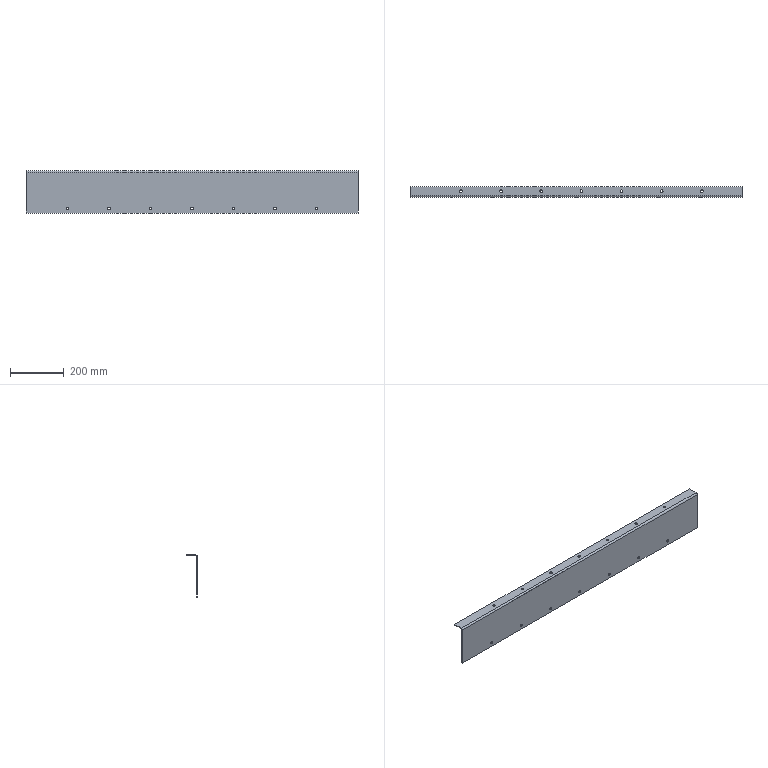Part | SolidWorks | features ICE 2, EdgeFlange 1, FlatPattern 1, SMBaseFlange 1, SheetMetal 1 | 1 solid | 42 faces | box 1240 x 40 x 157 mm | volume 711196 mm3 | cylinder 30 | plane 12 | commonest cylinder face diameters 10 x28 6 x1 12 x1
STEP:
#1=CARTESIAN_POINT('',(475.,20.,78.5));
#2=VERTEX_POINT('',#1);
#3=CARTESIAN_POINT('',(465.,20.,78.5));
#4=VERTEX_POINT('',#3);
#5=CARTESIAN_POINT('',(470.,20.,78.5));
#6=DIRECTION('',(0.,0.,-1.));
#7=DIRECTION('',(-1.,0.,0.));
#8=AXIS2_PLACEMENT_3D('',#5,#6,#7);
#9=CIRCLE('',#8,5.);
#10=EDGE_CURVE('',#2,#4,#9,.T.);
#11=ORIENTED_EDGE('',*,*,#10,.F.);
#12=CARTESIAN_POINT('',(475.,20.,75.5));
#13=VERTEX_POINT('',#12);
#14=CARTESIAN_POINT('',(475.,20.,255.5));
#15=DIRECTION('',(0.,0.,-1.));
#16=VECTOR('',#15,1000.);
#17=LINE('',#14,#16);
#18=EDGE_CURVE('',#2,#13,#17,.T.);
#19=ORIENTED_EDGE('',*,*,#18,.T.);
#20=CARTESIAN_POINT('',(465.,20.,75.5));
#21=VERTEX_POINT('',#20);
#22=CARTESIAN_POINT('',(470.,20.,75.5));
#23=DIRECTION('',(0.,0.,-1.));
#24=DIRECTION('',(-1.,0.,0.));
#25=AXIS2_PLACEMENT_3D('',#22,#23,#24);
#26=CIRCLE('',#25,5.);
#27=EDGE_CURVE('',#13,#21,#26,.T.);
#28=ORIENTED_EDGE('',*,*,#27,.T.);
#29=CARTESIAN_POINT('',(465.,20.,255.5));
#30=DIRECTION('',(0.,0.,-1.));
#31=VECTOR('',#30,1000.);
#32=LINE('',#29,#31);
#33=EDGE_CURVE('',#4,#21,#32,.T.);
#34=ORIENTED_EDGE('',*,*,#33,.F.);
#35=EDGE_LOOP('',(#11,#19,#28,#34));
#36=FACE_OUTER_BOUND('',#35,.T.);
#37=CARTESIAN_POINT('',(470.,20.,255.5));
#38=DIRECTION('',(0.,0.,-1.));
#39=DIRECTION('',(-1.,0.,0.));
#40=AXIS2_PLACEMENT_3D('',#37,#38,#39);
#41=CYLINDRICAL_SURFACE('',#40,5.);
#42=ADVANCED_FACE('',(#36),#41,.F.);
#43=CARTESIAN_POINT('',(325.,20.,78.5));
#44=VERTEX_POINT('',#43);
#45=CARTESIAN_POINT('',(315.,20.,78.5));
#46=VERTEX_POINT('',#45);
#47=CARTESIAN_POINT('',(320.,20.,78.5));
#48=DIRECTION('',(0.,0.,-1.));
#49=DIRECTION('',(-1.,0.,0.));
#50=AXIS2_PLACEMENT_3D('',#47,#48,#49);
#51=CIRCLE('',#50,5.);
#52=EDGE_CURVE('',#44,#46,#51,.T.);
#53=ORIENTED_EDGE('',*,*,#52,.F.);
#54=CARTESIAN_POINT('',(325.,20.,75.5));
#55=VERTEX_POINT('',#54);
#56=CARTESIAN_POINT('',(325.,20.,255.5));
#57=DIRECTION('',(0.,0.,-1.));
#58=VECTOR('',#57,1000.);
#59=LINE('',#56,#58);
#60=EDGE_CURVE('',#44,#55,#59,.T.);
#61=ORIENTED_EDGE('',*,*,#60,.T.);
#62=CARTESIAN_POINT('',(315.,20.,75.5));
#63=VERTEX_POINT('',#62);
#64=CARTESIAN_POINT('',(320.,20.,75.5));
#65=DIRECTION('',(0.,0.,-1.));
#66=DIRECTION('',(-1.,0.,0.));
#67=AXIS2_PLACEMENT_3D('',#64,#65,#66);
#68=CIRCLE('',#67,5.);
#69=EDGE_CURVE('',#55,#63,#68,.T.);
#70=ORIENTED_EDGE('',*,*,#69,.T.);
#71=CARTESIAN_POINT('',(315.,20.,255.5));
#72=DIRECTION('',(0.,0.,-1.));
#73=VECTOR('',#72,1000.);
#74=LINE('',#71,#73);
#75=EDGE_CURVE('',#46,#63,#74,.T.);
#76=ORIENTED_EDGE('',*,*,#75,.F.);
#77=EDGE_LOOP('',(#53,#61,#70,#76));
#78=FACE_OUTER_BOUND('',#77,.T.);
#79=CARTESIAN_POINT('',(320.,20.,255.5));
#80=DIRECTION('',(0.,0.,-1.));
#81=DIRECTION('',(-1.,0.,0.));
#82=AXIS2_PLACEMENT_3D('',#79,#80,#81);
#83=CYLINDRICAL_SURFACE('',#82,5.);
#84=ADVANCED_FACE('',(#78),#83,.F.);
#85=CARTESIAN_POINT('',(175.,20.,78.5));
#86=VERTEX_POINT('',#85);
#87=CARTESIAN_POINT('',(165.,20.,78.5));
#88=VERTEX_POINT('',#87);
#89=CARTESIAN_POINT('',(170.,20.,78.5));
#90=DIRECTION('',(0.,0.,-1.));
#91=DIRECTION('',(-1.,0.,0.));
#92=AXIS2_PLACEMENT_3D('',#89,#90,#91);
#93=CIRCLE('',#92,5.);
#94=EDGE_CURVE('',#86,#88,#93,.T.);
#95=ORIENTED_EDGE('',*,*,#94,.F.);
#96=CARTESIAN_POINT('',(175.,20.,75.5));
#97=VERTEX_POINT('',#96);
#98=CARTESIAN_POINT('',(175.,20.,255.5));
#99=DIRECTION('',(0.,0.,-1.));
#100=VECTOR('',#99,1000.);
#101=LINE('',#98,#100);
#102=EDGE_CURVE('',#86,#97,#101,.T.);
#103=ORIENTED_EDGE('',*,*,#102,.T.);
#104=CARTESIAN_POINT('',(165.,20.,75.5));
#105=VERTEX_POINT('',#104);
#106=CARTESIAN_POINT('',(170.,20.,75.5));
#107=DIRECTION('',(0.,0.,-1.));
#108=DIRECTION('',(-1.,0.,0.));
#109=AXIS2_PLACEMENT_3D('',#106,#107,#108);
#110=CIRCLE('',#109,5.);
#111=EDGE_CURVE('',#97,#105,#110,.T.);
#112=ORIENTED_EDGE('',*,*,#111,.T.);
#113=CARTESIAN_POINT('',(165.,20.,255.5));
#114=DIRECTION('',(0.,0.,-1.));
#115=VECTOR('',#114,1000.);
#116=LINE('',#113,#115);
#117=EDGE_CURVE('',#88,#105,#116,.T.);
#118=ORIENTED_EDGE('',*,*,#117,.F.);
#119=EDGE_LOOP('',(#95,#103,#112,#118));
#120=FACE_OUTER_BOUND('',#119,.T.);
#121=CARTESIAN_POINT('',(170.,20.,255.5));
#122=DIRECTION('',(0.,0.,-1.));
#123=DIRECTION('',(-1.,0.,0.));
#124=AXIS2_PLACEMENT_3D('',#121,#122,#123);
#125=CYLINDRICAL_SURFACE('',#124,5.);
#126=ADVANCED_FACE('',(#120),#125,.F.);
#127=CARTESIAN_POINT('',(25.,20.,78.5));
#128=VERTEX_POINT('',#127);
#129=CARTESIAN_POINT('',(15.,20.,78.5));
#130=VERTEX_POINT('',#129);
#131=CARTESIAN_POINT('',(20.,20.,78.5));
#132=DIRECTION('',(0.,0.,-1.));
#133=DIRECTION('',(-1.,0.,0.));
#134=AXIS2_PLACEMENT_3D('',#131,#132,#133);
#135=CIRCLE('',#134,5.);
#136=EDGE_CURVE('',#128,#130,#135,.T.);
#137=ORIENTED_EDGE('',*,*,#136,.F.);
#138=CARTESIAN_POINT('',(25.,20.,75.5));
#139=VERTEX_POINT('',#138);
#140=CARTESIAN_POINT('',(25.,20.,255.5));
#141=DIRECTION('',(0.,0.,-1.));
#142=VECTOR('',#141,1000.);
#143=LINE('',#140,#142);
#144=EDGE_CURVE('',#128,#139,#143,.T.);
#145=ORIENTED_EDGE('',*,*,#144,.T.);
#146=CARTESIAN_POINT('',(15.,20.,75.5));
#147=VERTEX_POINT('',#146);
#148=CARTESIAN_POINT('',(20.,20.,75.5));
#149=DIRECTION('',(0.,0.,-1.));
#150=DIRECTION('',(-1.,0.,0.));
#151=AXIS2_PLACEMENT_3D('',#148,#149,#150);
#152=CIRCLE('',#151,5.);
#153=EDGE_CURVE('',#139,#147,#152,.T.);
#154=ORIENTED_EDGE('',*,*,#153,.T.);
#155=CARTESIAN_POINT('',(15.,20.,255.5));
#156=DIRECTION('',(0.,0.,-1.));
#157=VECTOR('',#156,1000.);
#158=LINE('',#155,#157);
#159=EDGE_CURVE('',#130,#147,#158,.T.);
#160=ORIENTED_EDGE('',*,*,#159,.F.);
#161=EDGE_LOOP('',(#137,#145,#154,#160));
#162=FACE_OUTER_BOUND('',#161,.T.);
#163=CARTESIAN_POINT('',(20.,20.,255.5));
#164=DIRECTION('',(0.,0.,-1.));
#165=DIRECTION('',(-1.,0.,0.));
#166=AXIS2_PLACEMENT_3D('',#163,#164,#165);
#167=CYLINDRICAL_SURFACE('',#166,5.);
#168=ADVANCED_FACE('',(#162),#167,.F.);
#169=CARTESIAN_POINT('',(-125.,20.,78.5));
#170=VERTEX_POINT('',#169);
#171=CARTESIAN_POINT('',(-135.,20.,78.5));
#172=VERTEX_POINT('',#171);
#173=CARTESIAN_POINT('',(-130.,20.,78.5));
#174=DIRECTION('',(0.,0.,-1.));
#175=DIRECTION('',(-1.,0.,0.));
#176=AXIS2_PLACEMENT_3D('',#173,#174,#175);
#177=CIRCLE('',#176,5.);
#178=EDGE_CURVE('',#170,#172,#177,.T.);
#179=ORIENTED_EDGE('',*,*,#178,.F.);
#180=CARTESIAN_POINT('',(-125.,20.,75.5));
#181=VERTEX_POINT('',#180);
#182=CARTESIAN_POINT('',(-125.,20.,255.5));
#183=DIRECTION('',(0.,0.,-1.));
#184=VECTOR('',#183,1000.);
#185=LINE('',#182,#184);
#186=EDGE_CURVE('',#170,#181,#185,.T.);
#187=ORIENTED_EDGE('',*,*,#186,.T.);
#188=CARTESIAN_POINT('',(-135.,20.,75.5));
#189=VERTEX_POINT('',#188);
#190=CARTESIAN_POINT('',(-130.,20.,75.5));
#191=DIRECTION('',(0.,0.,-1.));
#192=DIRECTION('',(-1.,0.,0.));
#193=AXIS2_PLACEMENT_3D('',#190,#191,#192);
#194=CIRCLE('',#193,5.);
#195=EDGE_CURVE('',#181,#189,#194,.T.);
#196=ORIENTED_EDGE('',*,*,#195,.T.);
#197=CARTESIAN_POINT('',(-135.,20.,255.5));
#198=DIRECTION('',(0.,0.,-1.));
#199=VECTOR('',#198,1000.);
#200=LINE('',#197,#199);
#201=EDGE_CURVE('',#172,#189,#200,.T.);
#202=ORIENTED_EDGE('',*,*,#201,.F.);
#203=EDGE_LOOP('',(#179,#187,#196,#202));
#204=FACE_OUTER_BOUND('',#203,.T.);
#205=CARTESIAN_POINT('',(-130.,20.,255.5));
#206=DIRECTION('',(0.,0.,-1.));
#207=DIRECTION('',(-1.,0.,0.));
#208=AXIS2_PLACEMENT_3D('',#205,#206,#207);
#209=CYLINDRICAL_SURFACE('',#208,5.);
#210=ADVANCED_FACE('',(#204),#209,.F.);
#211=CARTESIAN_POINT('',(-275.,20.,78.5));
#212=VERTEX_POINT('',#211);
#213=CARTESIAN_POINT('',(-285.,20.,78.5));
#214=VERTEX_POINT('',#213);
#215=CARTESIAN_POINT('',(-280.,20.,78.5));
#216=DIRECTION('',(0.,0.,-1.));
#217=DIRECTION('',(-1.,0.,0.));
#218=AXIS2_PLACEMENT_3D('',#215,#216,#217);
#219=CIRCLE('',#218,5.);
#220=EDGE_CURVE('',#212,#214,#219,.T.);
#221=ORIENTED_EDGE('',*,*,#220,.F.);
#222=CARTESIAN_POINT('',(-275.,20.,75.5));
#223=VERTEX_POINT('',#222);
#224=CARTESIAN_POINT('',(-275.,20.,255.5));
#225=DIRECTION('',(0.,0.,-1.));
#226=VECTOR('',#225,1000.);
#227=LINE('',#224,#226);
#228=EDGE_CURVE('',#212,#223,#227,.T.);
#229=ORIENTED_EDGE('',*,*,#228,.T.);
#230=CARTESIAN_POINT('',(-285.,20.,75.5));
#231=VERTEX_POINT('',#230);
#232=CARTESIAN_POINT('',(-280.,20.,75.5));
#233=DIRECTION('',(0.,0.,-1.));
#234=DIRECTION('',(-1.,0.,0.));
#235=AXIS2_PLACEMENT_3D('',#232,#233,#234);
#236=CIRCLE('',#235,5.);
#237=EDGE_CURVE('',#223,#231,#236,.T.);
#238=ORIENTED_EDGE('',*,*,#237,.T.);
#239=CARTESIAN_POINT('',(-285.,20.,255.5));
#240=DIRECTION('',(0.,0.,-1.));
#241=VECTOR('',#240,1000.);
#242=LINE('',#239,#241);
#243=EDGE_CURVE('',#214,#231,#242,.T.);
#244=ORIENTED_EDGE('',*,*,#243,.F.);
#245=EDGE_LOOP('',(#221,#229,#238,#244));
#246=FACE_OUTER_BOUND('',#245,.T.);
#247=CARTESIAN_POINT('',(-280.,20.,255.5));
#248=DIRECTION('',(0.,0.,-1.));
#249=DIRECTION('',(-1.,0.,0.));
#250=AXIS2_PLACEMENT_3D('',#247,#248,#249);
#251=CYLINDRICAL_SURFACE('',#250,5.);
#252=ADVANCED_FACE('',(#246),#251,.F.);
#253=CARTESIAN_POINT('',(-425.,20.,78.5));
#254=VERTEX_POINT('',#253);
#255=CARTESIAN_POINT('',(-435.,20.,78.5));
#256=VERTEX_POINT('',#255);
#257=CARTESIAN_POINT('',(-430.,20.,78.5));
#258=DIRECTION('',(0.,0.,-1.));
#259=DIRECTION('',(-1.,0.,0.));
#260=AXIS2_PLACEMENT_3D('',#257,#258,#259);
#261=CIRCLE('',#260,5.);
#262=EDGE_CURVE('',#254,#256,#261,.T.);
#263=ORIENTED_EDGE('',*,*,#262,.F.);
#264=CARTESIAN_POINT('',(-425.,20.,75.5));
#265=VERTEX_POINT('',#264);
#266=CARTESIAN_POINT('',(-425.,20.,255.5));
#267=DIRECTION('',(0.,0.,-1.));
#268=VECTOR('',#267,1000.);
#269=LINE('',#266,#268);
#270=EDGE_CURVE('',#254,#265,#269,.T.);
#271=ORIENTED_EDGE('',*,*,#270,.T.);
#272=CARTESIAN_POINT('',(-435.,20.,75.5));
#273=VERTEX_POINT('',#272);
#274=CARTESIAN_POINT('',(-430.,20.,75.5));
#275=DIRECTION('',(0.,0.,-1.));
#276=DIRECTION('',(-1.,0.,0.));
#277=AXIS2_PLACEMENT_3D('',#274,#275,#276);
#278=CIRCLE('',#277,5.);
#279=EDGE_CURVE('',#265,#273,#278,.T.);
#280=ORIENTED_EDGE('',*,*,#279,.T.);
#281=CARTESIAN_POINT('',(-435.,20.,255.5));
#282=DIRECTION('',(0.,0.,-1.));
#283=VECTOR('',#282,1000.);
#284=LINE('',#281,#283);
#285=EDGE_CURVE('',#256,#273,#284,.T.);
#286=ORIENTED_EDGE('',*,*,#285,.F.);
#287=EDGE_LOOP('',(#263,#271,#280,#286));
#288=FACE_OUTER_BOUND('',#287,.T.);
#289=CARTESIAN_POINT('',(-430.,20.,255.5));
#290=DIRECTION('',(0.,0.,-1.));
#291=DIRECTION('',(-1.,0.,0.));
#292=AXIS2_PLACEMENT_3D('',#289,#290,#291);
#293=CYLINDRICAL_SURFACE('',#292,5.);
#294=ADVANCED_FACE('',(#288),#293,.F.);
#295=CARTESIAN_POINT('',(465.,-3.,-66.5));
#296=VERTEX_POINT('',#295);
#297=CARTESIAN_POINT('',(465.,-3.,-56.5));
#298=VERTEX_POINT('',#297);
#299=CARTESIAN_POINT('',(465.,-3.,-61.5));
#300=DIRECTION('',(0.,1.,0.));
#301=DIRECTION('',(0.,0.,1.));
#302=AXIS2_PLACEMENT_3D('',#299,#300,#301);
#303=CIRCLE('',#302,5.);
#304=EDGE_CURVE('',#296,#298,#303,.T.);
#305=ORIENTED_EDGE('',*,*,#304,.F.);
#306=CARTESIAN_POINT('',(465.,0.,-66.5));
#307=VERTEX_POINT('',#306);
#308=CARTESIAN_POINT('',(465.,-54.,-66.5));
#309=DIRECTION('',(0.,1.,0.));
#310=VECTOR('',#309,1000.);
#311=LINE('',#308,#310);
#312=EDGE_CURVE('',#296,#307,#311,.T.);
#313=ORIENTED_EDGE('',*,*,#312,.T.);
#314=CARTESIAN_POINT('',(465.,0.,-56.5));
#315=VERTEX_POINT('',#314);
#316=CARTESIAN_POINT('',(465.,0.,-61.5));
#317=DIRECTION('',(0.,1.,0.));
#318=DIRECTION('',(0.,0.,1.));
#319=AXIS2_PLACEMENT_3D('',#316,#317,#318);
#320=CIRCLE('',#319,5.);
#321=EDGE_CURVE('',#307,#315,#320,.T.);
#322=ORIENTED_EDGE('',*,*,#321,.T.);
#323=CARTESIAN_POINT('',(465.,-54.,-56.5));
#324=DIRECTION('',(0.,1.,0.));
#325=VECTOR('',#324,1000.);
#326=LINE('',#323,#325);
#327=EDGE_CURVE('',#298,#315,#326,.T.);
#328=ORIENTED_EDGE('',*,*,#327,.F.);
#329=EDGE_LOOP('',(#305,#313,#322,#328));
#330=FACE_OUTER_BOUND('',#329,.T.);
#331=CARTESIAN_POINT('',(465.,-54.,-61.5));
#332=DIRECTION('',(0.,1.,0.));
#333=DIRECTION('',(0.,0.,1.));
#334=AXIS2_PLACEMENT_3D('',#331,#332,#333);
#335=CYLINDRICAL_SURFACE('',#334,5.);
#336=ADVANCED_FACE('',(#330),#335,.F.);
#337=CARTESIAN_POINT('',(310.,-3.,-66.5));
#338=VERTEX_POINT('',#337);
#339=CARTESIAN_POINT('',(310.,-3.,-56.5));
#340=VERTEX_POINT('',#339);
#341=CARTESIAN_POINT('',(310.,-3.,-61.5));
#342=DIRECTION('',(0.,1.,0.));
#343=DIRECTION('',(0.,0.,1.));
#344=AXIS2_PLACEMENT_3D('',#341,#342,#343);
#345=CIRCLE('',#344,5.);
#346=EDGE_CURVE('',#338,#340,#345,.T.);
#347=ORIENTED_EDGE('',*,*,#346,.F.);
#348=CARTESIAN_POINT('',(310.,0.,-66.5));
#349=VERTEX_POINT('',#348);
#350=CARTESIAN_POINT('',(310.,-54.,-66.5));
#351=DIRECTION('',(0.,1.,0.));
#352=VECTOR('',#351,1000.);
#353=LINE('',#350,#352);
#354=EDGE_CURVE('',#338,#349,#353,.T.);
#355=ORIENTED_EDGE('',*,*,#354,.T.);
#356=CARTESIAN_POINT('',(310.,0.,-56.5));
#357=VERTEX_POINT('',#356);
#358=CARTESIAN_POINT('',(310.,0.,-61.5));
#359=DIRECTION('',(0.,1.,0.));
#360=DIRECTION('',(0.,0.,1.));
#361=AXIS2_PLACEMENT_3D('',#358,#359,#360);
#362=CIRCLE('',#361,5.);
#363=EDGE_CURVE('',#349,#357,#362,.T.);
#364=ORIENTED_EDGE('',*,*,#363,.T.);
#365=CARTESIAN_POINT('',(310.,-54.,-56.5));
#366=DIRECTION('',(0.,1.,0.));
#367=VECTOR('',#366,1000.);
#368=LINE('',#365,#367);
#369=EDGE_CURVE('',#340,#357,#368,.T.);
#370=ORIENTED_EDGE('',*,*,#369,.F.);
#371=EDGE_LOOP('',(#347,#355,#364,#370));
#372=FACE_OUTER_BOUND('',#371,.T.);
#373=CARTESIAN_POINT('',(310.,-54.,-61.5));
#374=DIRECTION('',(0.,1.,0.));
#375=DIRECTION('',(0.,0.,1.));
#376=AXIS2_PLACEMENT_3D('',#373,#374,#375);
#377=CYLINDRICAL_SURFACE('',#376,5.);
#378=ADVANCED_FACE('',(#372),#377,.F.);
#379=CARTESIAN_POINT('',(155.,-3.,-66.5));
#380=VERTEX_POINT('',#379);
#381=CARTESIAN_POINT('',(155.,-3.,-56.5));
#382=VERTEX_POINT('',#381);
#383=CARTESIAN_POINT('',(155.,-3.,-61.5));
#384=DIRECTION('',(0.,1.,0.));
#385=DIRECTION('',(0.,0.,1.));
#386=AXIS2_PLACEMENT_3D('',#383,#384,#385);
#387=CIRCLE('',#386,5.);
#388=EDGE_CURVE('',#380,#382,#387,.T.);
#389=ORIENTED_EDGE('',*,*,#388,.F.);
#390=CARTESIAN_POINT('',(155.,0.,-66.5));
#391=VERTEX_POINT('',#390);
#392=CARTESIAN_POINT('',(155.,-54.,-66.5));
#393=DIRECTION('',(0.,1.,0.));
#394=VECTOR('',#393,1000.);
#395=LINE('',#392,#394);
#396=EDGE_CURVE('',#380,#391,#395,.T.);
#397=ORIENTED_EDGE('',*,*,#396,.T.);
#398=CARTESIAN_POINT('',(155.,0.,-56.5));
#399=VERTEX_POINT('',#398);
#400=CARTESIAN_POINT('',(155.,0.,-61.5));
#401=DIRECTION('',(0.,1.,0.));
#402=DIRECTION('',(0.,0.,1.));
#403=AXIS2_PLACEMENT_3D('',#400,#401,#402);
#404=CIRCLE('',#403,5.);
#405=EDGE_CURVE('',#391,#399,#404,.T.);
#406=ORIENTED_EDGE('',*,*,#405,.T.);
#407=CARTESIAN_POINT('',(155.,-54.,-56.5));
#408=DIRECTION('',(0.,1.,0.));
#409=VECTOR('',#408,1000.);
#410=LINE('',#407,#409);
#411=EDGE_CURVE('',#382,#399,#410,.T.);
#412=ORIENTED_EDGE('',*,*,#411,.F.);
#413=EDGE_LOOP('',(#389,#397,#406,#412));
#414=FACE_OUTER_BOUND('',#413,.T.);
#415=CARTESIAN_POINT('',(155.,-54.,-61.5));
#416=DIRECTION('',(0.,1.,0.));
#417=DIRECTION('',(0.,0.,1.));
#418=AXIS2_PLACEMENT_3D('',#415,#416,#417);
#419=CYLINDRICAL_SURFACE('',#418,5.);
#420=ADVANCED_FACE('',(#414),#419,.F.);
#421=CARTESIAN_POINT('',(0.,-3.,-66.5));
#422=VERTEX_POINT('',#421);
#423=CARTESIAN_POINT('',(0.,-3.,-56.5));
#424=VERTEX_POINT('',#423);
#425=CARTESIAN_POINT('',(0.,-3.,-61.5));
#426=DIRECTION('',(0.,1.,0.));
#427=DIRECTION('',(0.,0.,1.));
#428=AXIS2_PLACEMENT_3D('',#425,#426,#427);
#429=CIRCLE('',#428,5.);
#430=EDGE_CURVE('',#422,#424,#429,.T.);
#431=ORIENTED_EDGE('',*,*,#430,.F.);
#432=CARTESIAN_POINT('',(0.,0.,-66.5));
#433=VERTEX_POINT('',#432);
#434=CARTESIAN_POINT('',(0.,-54.,-66.5));
#435=DIRECTION('',(0.,1.,0.));
#436=VECTOR('',#435,1000.);
#437=LINE('',#434,#436);
#438=EDGE_CURVE('',#422,#433,#437,.T.);
#439=ORIENTED_EDGE('',*,*,#438,.T.);
#440=CARTESIAN_POINT('',(0.,0.,-56.5));
#441=VERTEX_POINT('',#440);
#442=CARTESIAN_POINT('',(0.,0.,-61.5));
#443=DIRECTION('',(0.,1.,0.));
#444=DIRECTION('',(0.,0.,1.));
#445=AXIS2_PLACEMENT_3D('',#442,#443,#444);
#446=CIRCLE('',#445,5.);
#447=EDGE_CURVE('',#433,#441,#446,.T.);
#448=ORIENTED_EDGE('',*,*,#447,.T.);
#449=CARTESIAN_POINT('',(0.,-54.,-56.5));
#450=DIRECTION('',(0.,1.,0.));
#451=VECTOR('',#450,1000.);
#452=LINE('',#449,#451);
#453=EDGE_CURVE('',#424,#441,#452,.T.);
#454=ORIENTED_EDGE('',*,*,#453,.F.);
#455=EDGE_LOOP('',(#431,#439,#448,#454));
#456=FACE_OUTER_BOUND('',#455,.T.);
#457=CARTESIAN_POINT('',(0.,-54.,-61.5));
#458=DIRECTION('',(0.,1.,0.));
#459=DIRECTION('',(0.,0.,1.));
#460=AXIS2_PLACEMENT_3D('',#457,#458,#459);
#461=CYLINDRICAL_SURFACE('',#460,5.);
#462=ADVANCED_FACE('',(#456),#461,.F.);
#463=CARTESIAN_POINT('',(-155.,-3.,-66.5));
#464=VERTEX_POINT('',#463);
#465=CARTESIAN_POINT('',(-155.,-3.,-56.5));
#466=VERTEX_POINT('',#465);
#467=CARTESIAN_POINT('',(-155.,-3.,-61.5));
#468=DIRECTION('',(0.,1.,0.));
#469=DIRECTION('',(0.,0.,1.));
#470=AXIS2_PLACEMENT_3D('',#467,#468,#469);
#471=CIRCLE('',#470,5.);
#472=EDGE_CURVE('',#464,#466,#471,.T.);
#473=ORIENTED_EDGE('',*,*,#472,.F.);
#474=CARTESIAN_POINT('',(-155.,0.,-66.5));
#475=VERTEX_POINT('',#474);
#476=CARTESIAN_POINT('',(-155.,-54.,-66.5));
#477=DIRECTION('',(0.,1.,0.));
#478=VECTOR('',#477,1000.);
#479=LINE('',#476,#478);
#480=EDGE_CURVE('',#464,#475,#479,.T.);
#481=ORIENTED_EDGE('',*,*,#480,.T.);
#482=CARTESIAN_POINT('',(-155.,0.,-56.5));
#483=VERTEX_POINT('',#482);
#484=CARTESIAN_POINT('',(-155.,0.,-61.5));
#485=DIRECTION('',(0.,1.,0.));
#486=DIRECTION('',(0.,0.,1.));
#487=AXIS2_PLACEMENT_3D('',#484,#485,#486);
#488=CIRCLE('',#487,5.);
#489=EDGE_CURVE('',#475,#483,#488,.T.);
#490=ORIENTED_EDGE('',*,*,#489,.T.);
#491=CARTESIAN_POINT('',(-155.,-54.,-56.5));
#492=DIRECTION('',(0.,1.,0.));
#493=VECTOR('',#492,1000.);
#494=LINE('',#491,#493);
#495=EDGE_CURVE('',#466,#483,#494,.T.);
#496=ORIENTED_EDGE('',*,*,#495,.F.);
#497=EDGE_LOOP('',(#473,#481,#490,#496));
#498=FACE_OUTER_BOUND('',#497,.T.);
#499=CARTESIAN_POINT('',(-155.,-54.,-61.5));
#500=DIRECTION('',(0.,1.,0.));
#501=DIRECTION('',(0.,0.,1.));
#502=AXIS2_PLACEMENT_3D('',#499,#500,#501);
#503=CYLINDRICAL_SURFACE('',#502,5.);
#504=ADVANCED_FACE('',(#498),#503,.F.);
#505=CARTESIAN_POINT('',(-310.,-3.,-66.5));
#506=VERTEX_POINT('',#505);
#507=CARTESIAN_POINT('',(-310.,-3.,-56.5));
#508=VERTEX_POINT('',#507);
#509=CARTESIAN_POINT('',(-310.,-3.,-61.5));
#510=DIRECTION('',(0.,1.,0.));
#511=DIRECTION('',(0.,0.,1.));
#512=AXIS2_PLACEMENT_3D('',#509,#510,#511);
#513=CIRCLE('',#512,5.);
#514=EDGE_CURVE('',#506,#508,#513,.T.);
#515=ORIENTED_EDGE('',*,*,#514,.F.);
#516=CARTESIAN_POINT('',(-310.,0.,-66.5));
#517=VERTEX_POINT('',#516);
#518=CARTESIAN_POINT('',(-310.,-54.,-66.5));
#519=DIRECTION('',(0.,1.,0.));
#520=VECTOR('',#519,1000.);
#521=LINE('',#518,#520);
#522=EDGE_CURVE('',#506,#517,#521,.T.);
#523=ORIENTED_EDGE('',*,*,#522,.T.);
#524=CARTESIAN_POINT('',(-310.,0.,-56.5));
#525=VERTEX_POINT('',#524);
#526=CARTESIAN_POINT('',(-310.,0.,-61.5));
#527=DIRECTION('',(0.,1.,0.));
#528=DIRECTION('',(0.,0.,1.));
#529=AXIS2_PLACEMENT_3D('',#526,#527,#528);
#530=CIRCLE('',#529,5.);
#531=EDGE_CURVE('',#517,#525,#530,.T.);
#532=ORIENTED_EDGE('',*,*,#531,.T.);
#533=CARTESIAN_POINT('',(-310.,-54.,-56.5));
#534=DIRECTION('',(0.,1.,0.));
#535=VECTOR('',#534,1000.);
#536=LINE('',#533,#535);
#537=EDGE_CURVE('',#508,#525,#536,.T.);
#538=ORIENTED_EDGE('',*,*,#537,.F.);
#539=EDGE_LOOP('',(#515,#523,#532,#538));
#540=FACE_OUTER_BOUND('',#539,.T.);
#541=CARTESIAN_POINT('',(-310.,-54.,-61.5));
#542=DIRECTION('',(0.,1.,0.));
#543=DIRECTION('',(0.,0.,1.));
#544=AXIS2_PLACEMENT_3D('',#541,#542,#543);
#545=CYLINDRICAL_SURFACE('',#544,5.);
#546=ADVANCED_FACE('',(#540),#545,.F.);
#547=CARTESIAN_POINT('',(-465.,-3.,-66.5));
#548=VERTEX_POINT('',#547);
#549=CARTESIAN_POINT('',(-465.,-3.,-56.5));
#550=VERTEX_POINT('',#549);
#551=CARTESIAN_POINT('',(-465.,-3.,-61.5));
#552=DIRECTION('',(0.,1.,0.));
#553=DIRECTION('',(0.,0.,1.));
#554=AXIS2_PLACEMENT_3D('',#551,#552,#553);
#555=CIRCLE('',#554,5.);
#556=EDGE_CURVE('',#548,#550,#555,.T.);
#557=ORIENTED_EDGE('',*,*,#556,.F.);
#558=CARTESIAN_POINT('',(-465.,0.,-66.5));
#559=VERTEX_POINT('',#558);
#560=CARTESIAN_POINT('',(-465.,-54.,-66.5));
#561=DIRECTION('',(0.,1.,0.));
#562=VECTOR('',#561,1000.);
#563=LINE('',#560,#562);
#564=EDGE_CURVE('',#548,#559,#563,.T.);
#565=ORIENTED_EDGE('',*,*,#564,.T.);
#566=CARTESIAN_POINT('',(-465.,0.,-56.5));
#567=VERTEX_POINT('',#566);
#568=CARTESIAN_POINT('',(-465.,0.,-61.5));
#569=DIRECTION('',(0.,1.,0.));
#570=DIRECTION('',(0.,0.,1.));
#571=AXIS2_PLACEMENT_3D('',#568,#569,#570);
#572=CIRCLE('',#571,5.);
#573=EDGE_CURVE('',#559,#567,#572,.T.);
#574=ORIENTED_EDGE('',*,*,#573,.T.);
#575=CARTESIAN_POINT('',(-465.,-54.,-56.5));
#576=DIRECTION('',(0.,1.,0.));
#577=VECTOR('',#576,1000.);
#578=LINE('',#575,#577);
#579=EDGE_CURVE('',#550,#567,#578,.T.);
#580=ORIENTED_EDGE('',*,*,#579,.F.);
#581=EDGE_LOOP('',(#557,#565,#574,#580));
#582=FACE_OUTER_BOUND('',#581,.T.);
#583=CARTESIAN_POINT('',(-465.,-54.,-61.5));
#584=DIRECTION('',(0.,1.,0.));
#585=DIRECTION('',(0.,0.,1.));
#586=AXIS2_PLACEMENT_3D('',#583,#584,#585);
#587=CYLINDRICAL_SURFACE('',#586,5.);
#588=ADVANCED_FACE('',(#582),#587,.F.);
#589=CARTESIAN_POINT('',(620.,0.,72.5));
#590=VERTEX_POINT('',#589);
#591=CARTESIAN_POINT('',(620.,0.,-78.5));
#592=VERTEX_POINT('',#591);
#593=CARTESIAN_POINT('',(620.,0.,-78.5));
#594=DIRECTION('',(0.,0.,-1.));
#595=VECTOR('',#594,1000.);
#596=LINE('',#593,#595);
#597=EDGE_CURVE('',#590,#592,#596,.T.);
#598=ORIENTED_EDGE('',*,*,#597,.F.);
#599=CARTESIAN_POINT('',(620.,-3.,72.5));
#600=VERTEX_POINT('',#599);
#601=CARTESIAN_POINT('',(620.,0.,72.5));
#602=DIRECTION('',(0.,-1.,0.));
#603=VECTOR('',#602,1000.);
#604=LINE('',#601,#603);
#605=EDGE_CURVE('',#590,#600,#604,.T.);
#606=ORIENTED_EDGE('',*,*,#605,.T.);
#607=CARTESIAN_POINT('',(620.,-3.,-78.5));
#608=VERTEX_POINT('',#607);
#609=CARTESIAN_POINT('',(620.,-3.,-78.5));
#610=DIRECTION('',(0.,0.,-1.));
#611=VECTOR('',#610,1000.);
#612=LINE('',#609,#611);
#613=EDGE_CURVE('',#600,#608,#612,.T.);
#614=ORIENTED_EDGE('',*,*,#613,.T.);
#615=CARTESIAN_POINT('',(620.,-3.,-78.5));
#616=DIRECTION('',(0.,1.,0.));
#617=VECTOR('',#616,1000.);
#618=LINE('',#615,#617);
#619=EDGE_CURVE('',#608,#592,#618,.T.);
#620=ORIENTED_EDGE('',*,*,#619,.T.);
#621=EDGE_LOOP('',(#598,#606,#614,#620));
#622=FACE_OUTER_BOUND('',#621,.T.);
#623=CARTESIAN_POINT('',(620.,-3.,-78.5));
#624=DIRECTION('',(1.,0.,0.));
#625=DIRECTION('',(0.,0.,-1.));
#626=AXIS2_PLACEMENT_3D('',#623,#624,#625);
#627=PLANE('',#626);
#628=ADVANCED_FACE('',(#622),#627,.T.);
#629=CARTESIAN_POINT('',(465.,-3.,-61.5));
#630=DIRECTION('',(0.,1.,0.));
#631=DIRECTION('',(0.,0.,1.));
#632=AXIS2_PLACEMENT_3D('',#629,#630,#631);
#633=CIRCLE('',#632,5.);
#634=EDGE_CURVE('',#298,#296,#633,.T.);
#635=ORIENTED_EDGE('',*,*,#634,.T.);
#636=ORIENTED_EDGE('',*,*,#304,.T.);
#637=EDGE_LOOP('',(#635,#636));
#638=FACE_BOUND('',#637,.T.);
#639=CARTESIAN_POINT('',(310.,-3.,-61.5));
#640=DIRECTION('',(0.,1.,0.));
#641=DIRECTION('',(0.,0.,1.));
#642=AXIS2_PLACEMENT_3D('',#639,#640,#641);
#643=CIRCLE('',#642,5.);
#644=EDGE_CURVE('',#340,#338,#643,.T.);
#645=ORIENTED_EDGE('',*,*,#644,.T.);
#646=ORIENTED_EDGE('',*,*,#346,.T.);
#647=EDGE_LOOP('',(#645,#646));
#648=FACE_BOUND('',#647,.T.);
#649=CARTESIAN_POINT('',(155.,-3.,-61.5));
#650=DIRECTION('',(0.,1.,0.));
#651=DIRECTION('',(0.,0.,1.));
#652=AXIS2_PLACEMENT_3D('',#649,#650,#651);
#653=CIRCLE('',#652,5.);
#654=EDGE_CURVE('',#382,#380,#653,.T.);
#655=ORIENTED_EDGE('',*,*,#654,.T.);
#656=ORIENTED_EDGE('',*,*,#388,.T.);
#657=EDGE_LOOP('',(#655,#656));
#658=FACE_BOUND('',#657,.T.);
#659=CARTESIAN_POINT('',(0.,-3.,-61.5));
#660=DIRECTION('',(0.,1.,0.));
#661=DIRECTION('',(0.,0.,1.));
#662=AXIS2_PLACEMENT_3D('',#659,#660,#661);
#663=CIRCLE('',#662,5.);
#664=EDGE_CURVE('',#424,#422,#663,.T.);
#665=ORIENTED_EDGE('',*,*,#664,.T.);
#666=ORIENTED_EDGE('',*,*,#430,.T.);
#667=EDGE_LOOP('',(#665,#666));
#668=FACE_BOUND('',#667,.T.);
#669=CARTESIAN_POINT('',(-155.,-3.,-61.5));
#670=DIRECTION('',(0.,1.,0.));
#671=DIRECTION('',(0.,0.,1.));
#672=AXIS2_PLACEMENT_3D('',#669,#670,#671);
#673=CIRCLE('',#672,5.);
#674=EDGE_CURVE('',#466,#464,#673,.T.);
#675=ORIENTED_EDGE('',*,*,#674,.T.);
#676=ORIENTED_EDGE('',*,*,#472,.T.);
#677=EDGE_LOOP('',(#675,#676));
#678=FACE_BOUND('',#677,.T.);
#679=CARTESIAN_POINT('',(-310.,-3.,-61.5));
#680=DIRECTION('',(0.,1.,0.));
#681=DIRECTION('',(0.,0.,1.));
#682=AXIS2_PLACEMENT_3D('',#679,#680,#681);
#683=CIRCLE('',#682,5.);
#684=EDGE_CURVE('',#508,#506,#683,.T.);
#685=ORIENTED_EDGE('',*,*,#684,.T.);
#686=ORIENTED_EDGE('',*,*,#514,.T.);
#687=EDGE_LOOP('',(#685,#686));
#688=FACE_BOUND('',#687,.T.);
#689=CARTESIAN_POINT('',(-465.,-3.,-61.5));
#690=DIRECTION('',(0.,1.,0.));
#691=DIRECTION('',(0.,0.,1.));
#692=AXIS2_PLACEMENT_3D('',#689,#690,#691);
#693=CIRCLE('',#692,5.);
#694=EDGE_CURVE('',#550,#548,#693,.T.);
#695=ORIENTED_EDGE('',*,*,#694,.T.);
#696=ORIENTED_EDGE('',*,*,#556,.T.);
#697=EDGE_LOOP('',(#695,#696));
#698=FACE_BOUND('',#697,.T.);
#699=CARTESIAN_POINT('',(-620.,-3.,72.5));
#700=VERTEX_POINT('',#699);
#701=CARTESIAN_POINT('',(620.,-3.,72.5));
#702=DIRECTION('',(-1.,0.,0.));
#703=VECTOR('',#702,1000.);
#704=LINE('',#701,#703);
#705=EDGE_CURVE('',#600,#700,#704,.T.);
#706=ORIENTED_EDGE('',*,*,#705,.T.);
#707=CARTESIAN_POINT('',(-620.,-3.,-78.5));
#708=VERTEX_POINT('',#707);
#709=CARTESIAN_POINT('',(-620.,-3.,-78.5));
#710=DIRECTION('',(0.,0.,1.));
#711=VECTOR('',#710,1000.);
#712=LINE('',#709,#711);
#713=EDGE_CURVE('',#708,#700,#712,.T.);
#714=ORIENTED_EDGE('',*,*,#713,.F.);
#715=CARTESIAN_POINT('',(-620.,-3.,-78.5));
#716=DIRECTION('',(-1.,0.,0.));
#717=VECTOR('',#716,1000.);
#718=LINE('',#715,#717);
#719=EDGE_CURVE('',#608,#708,#718,.T.);
#720=ORIENTED_EDGE('',*,*,#719,.F.);
#721=ORIENTED_EDGE('',*,*,#613,.F.);
#722=EDGE_LOOP('',(#706,#714,#720,#721));
#723=FACE_OUTER_BOUND('',#722,.T.);
#724=CARTESIAN_POINT('',(0.,-3.,0.));
#725=DIRECTION('',(0.,1.,0.));
#726=DIRECTION('',(0.,0.,1.));
#727=AXIS2_PLACEMENT_3D('',#724,#725,#726);
#728=PLANE('',#727);
#729=ADVANCED_FACE('',(#638,#648,#658,#668,#678,#688,#698,#723),#728,.F.);
#730=CARTESIAN_POINT('',(465.,0.,-61.5));
#731=DIRECTION('',(0.,1.,0.));
#732=DIRECTION('',(0.,0.,1.));
#733=AXIS2_PLACEMENT_3D('',#730,#731,#732);
#734=CIRCLE('',#733,5.);
#735=EDGE_CURVE('',#315,#307,#734,.T.);
#736=ORIENTED_EDGE('',*,*,#735,.F.);
#737=ORIENTED_EDGE('',*,*,#321,.F.);
#738=EDGE_LOOP('',(#736,#737));
#739=FACE_BOUND('',#738,.T.);
#740=CARTESIAN_POINT('',(310.,0.,-61.5));
#741=DIRECTION('',(0.,1.,0.));
#742=DIRECTION('',(0.,0.,1.));
#743=AXIS2_PLACEMENT_3D('',#740,#741,#742);
#744=CIRCLE('',#743,5.);
#745=EDGE_CURVE('',#357,#349,#744,.T.);
#746=ORIENTED_EDGE('',*,*,#745,.F.);
#747=ORIENTED_EDGE('',*,*,#363,.F.);
#748=EDGE_LOOP('',(#746,#747));
#749=FACE_BOUND('',#748,.T.);
#750=CARTESIAN_POINT('',(155.,0.,-61.5));
#751=DIRECTION('',(0.,1.,0.));
#752=DIRECTION('',(0.,0.,1.));
#753=AXIS2_PLACEMENT_3D('',#750,#751,#752);
#754=CIRCLE('',#753,5.);
#755=EDGE_CURVE('',#399,#391,#754,.T.);
#756=ORIENTED_EDGE('',*,*,#755,.F.);
#757=ORIENTED_EDGE('',*,*,#405,.F.);
#758=EDGE_LOOP('',(#756,#757));
#759=FACE_BOUND('',#758,.T.);
#760=CARTESIAN_POINT('',(0.,0.,-61.5));
#761=DIRECTION('',(0.,1.,0.));
#762=DIRECTION('',(0.,0.,1.));
#763=AXIS2_PLACEMENT_3D('',#760,#761,#762);
#764=CIRCLE('',#763,5.);
#765=EDGE_CURVE('',#441,#433,#764,.T.);
#766=ORIENTED_EDGE('',*,*,#765,.F.);
#767=ORIENTED_EDGE('',*,*,#447,.F.);
#768=EDGE_LOOP('',(#766,#767));
#769=FACE_BOUND('',#768,.T.);
#770=CARTESIAN_POINT('',(-155.,0.,-61.5));
#771=DIRECTION('',(0.,1.,0.));
#772=DIRECTION('',(0.,0.,1.));
#773=AXIS2_PLACEMENT_3D('',#770,#771,#772);
#774=CIRCLE('',#773,5.);
#775=EDGE_CURVE('',#483,#475,#774,.T.);
#776=ORIENTED_EDGE('',*,*,#775,.F.);
#777=ORIENTED_EDGE('',*,*,#489,.F.);
#778=EDGE_LOOP('',(#776,#777));
#779=FACE_BOUND('',#778,.T.);
#780=CARTESIAN_POINT('',(-310.,0.,-61.5));
#781=DIRECTION('',(0.,1.,0.));
#782=DIRECTION('',(0.,0.,1.));
#783=AXIS2_PLACEMENT_3D('',#780,#781,#782);
#784=CIRCLE('',#783,5.);
#785=EDGE_CURVE('',#525,#517,#784,.T.);
#786=ORIENTED_EDGE('',*,*,#785,.F.);
#787=ORIENTED_EDGE('',*,*,#531,.F.);
#788=EDGE_LOOP('',(#786,#787));
#789=FACE_BOUND('',#788,.T.);
#790=CARTESIAN_POINT('',(-465.,0.,-61.5));
#791=DIRECTION('',(0.,1.,0.));
#792=DIRECTION('',(0.,0.,1.));
#793=AXIS2_PLACEMENT_3D('',#790,#791,#792);
#794=CIRCLE('',#793,5.);
#795=EDGE_CURVE('',#567,#559,#794,.T.);
#796=ORIENTED_EDGE('',*,*,#795,.F.);
#797=ORIENTED_EDGE('',*,*,#573,.F.);
#798=EDGE_LOOP('',(#796,#797));
#799=FACE_BOUND('',#798,.T.);
#800=CARTESIAN_POINT('',(-620.,0.,-78.5));
#801=VERTEX_POINT('',#800);
#802=CARTESIAN_POINT('',(-620.,0.,72.5));
#803=VERTEX_POINT('',#802);
#804=CARTESIAN_POINT('',(-620.,0.,-78.5));
#805=DIRECTION('',(0.,0.,1.));
#806=VECTOR('',#805,1000.);
#807=LINE('',#804,#806);
#808=EDGE_CURVE('',#801,#803,#807,.T.);
#809=ORIENTED_EDGE('',*,*,#808,.T.);
#810=CARTESIAN_POINT('',(620.,0.,72.5));
#811=DIRECTION('',(-1.,0.,0.));
#812=VECTOR('',#811,1000.);
#813=LINE('',#810,#812);
#814=EDGE_CURVE('',#590,#803,#813,.T.);
#815=ORIENTED_EDGE('',*,*,#814,.F.);
#816=ORIENTED_EDGE('',*,*,#597,.T.);
#817=CARTESIAN_POINT('',(-620.,0.,-78.5));
#818=DIRECTION('',(-1.,0.,0.));
#819=VECTOR('',#818,1000.);
#820=LINE('',#817,#819);
#821=EDGE_CURVE('',#592,#801,#820,.T.);
#822=ORIENTED_EDGE('',*,*,#821,.T.);
#823=EDGE_LOOP('',(#809,#815,#816,#822));
#824=FACE_OUTER_BOUND('',#823,.T.);
#825=CARTESIAN_POINT('',(0.,0.,0.));
#826=DIRECTION('',(0.,1.,0.));
#827=DIRECTION('',(0.,0.,1.));
#828=AXIS2_PLACEMENT_3D('',#825,#826,#827);
#829=PLANE('',#828);
#830=ADVANCED_FACE('',(#739,#749,#759,#769,#779,#789,#799,#824),#829,.T.);
#831=CARTESIAN_POINT('',(-620.,0.,72.5));
#832=DIRECTION('',(0.,-1.,0.));
#833=VECTOR('',#832,1000.);
#834=LINE('',#831,#833);
#835=EDGE_CURVE('',#803,#700,#834,.T.);
#836=ORIENTED_EDGE('',*,*,#835,.F.);
#837=ORIENTED_EDGE('',*,*,#808,.F.);
#838=CARTESIAN_POINT('',(-620.,-3.,-78.5));
#839=DIRECTION('',(0.,1.,0.));
#840=VECTOR('',#839,1000.);
#841=LINE('',#838,#840);
#842=EDGE_CURVE('',#708,#801,#841,.T.);
#843=ORIENTED_EDGE('',*,*,#842,.F.);
#844=ORIENTED_EDGE('',*,*,#713,.T.);
#845=EDGE_LOOP('',(#836,#837,#843,#844));
#846=FACE_OUTER_BOUND('',#845,.T.);
#847=CARTESIAN_POINT('',(-620.,-3.,-78.5));
#848=DIRECTION('',(-1.,0.,0.));
#849=DIRECTION('',(0.,0.,1.));
#850=AXIS2_PLACEMENT_3D('',#847,#848,#849);
#851=PLANE('',#850);
#852=ADVANCED_FACE('',(#846),#851,.T.);
#853=ORIENTED_EDGE('',*,*,#821,.F.);
#854=ORIENTED_EDGE('',*,*,#619,.F.);
#855=ORIENTED_EDGE('',*,*,#719,.T.);
#856=ORIENTED_EDGE('',*,*,#842,.T.);
#857=EDGE_LOOP('',(#853,#854,#855,#856));
#858=FACE_OUTER_BOUND('',#857,.T.);
#859=CARTESIAN_POINT('',(-620.,-3.,-78.5));
#860=DIRECTION('',(0.,0.,-1.));
#861=DIRECTION('',(-1.,0.,0.));
#862=AXIS2_PLACEMENT_3D('',#859,#860,#861);
#863=PLANE('',#862);
#864=ADVANCED_FACE('',(#858),#863,.T.);
#865=CARTESIAN_POINT('',(-620.,3.,75.5));
#866=VERTEX_POINT('',#865);
#867=CARTESIAN_POINT('',(-620.,3.,78.5));
#868=VERTEX_POINT('',#867);
#869=CARTESIAN_POINT('',(-620.,3.,78.5));
#870=DIRECTION('',(0.,0.,1.));
#871=VECTOR('',#870,1000.);
#872=LINE('',#869,#871);
#873=EDGE_CURVE('',#866,#868,#872,.T.);
#874=ORIENTED_EDGE('',*,*,#873,.F.);
#875=CARTESIAN_POINT('',(-620.,3.,72.5));
#876=DIRECTION('',(-1.,0.,0.));
#877=DIRECTION('',(0.,0.,-1.));
#878=AXIS2_PLACEMENT_3D('',#875,#876,#877);
#879=CIRCLE('',#878,3.);
#880=EDGE_CURVE('',#803,#866,#879,.T.);
#881=ORIENTED_EDGE('',*,*,#880,.F.);
#882=ORIENTED_EDGE('',*,*,#835,.T.);
#883=CARTESIAN_POINT('',(-620.,3.,72.5));
#884=DIRECTION('',(-1.,0.,0.));
#885=DIRECTION('',(0.,0.,-1.));
#886=AXIS2_PLACEMENT_3D('',#883,#884,#885);
#887=CIRCLE('',#886,6.);
#888=EDGE_CURVE('',#700,#868,#887,.T.);
#889=ORIENTED_EDGE('',*,*,#888,.T.);
#890=EDGE_LOOP('',(#874,#881,#882,#889));
#891=FACE_OUTER_BOUND('',#890,.T.);
#892=CARTESIAN_POINT('',(-620.,3.,72.5));
#893=DIRECTION('',(-1.,0.,0.));
#894=DIRECTION('',(0.,0.,1.));
#895=AXIS2_PLACEMENT_3D('',#892,#893,#894);
#896=PLANE('',#895);
#897=ADVANCED_FACE('',(#891),#896,.T.);
#898=CARTESIAN_POINT('',(620.,3.,75.5));
#899=VERTEX_POINT('',#898);
#900=CARTESIAN_POINT('',(620.,3.,72.5));
#901=DIRECTION('',(1.,0.,0.));
#902=DIRECTION('',(0.,0.,-1.));
#903=AXIS2_PLACEMENT_3D('',#900,#901,#902);
#904=CIRCLE('',#903,3.);
#905=EDGE_CURVE('',#899,#590,#904,.T.);
#906=ORIENTED_EDGE('',*,*,#905,.F.);
#907=CARTESIAN_POINT('',(620.,3.,78.5));
#908=VERTEX_POINT('',#907);
#909=CARTESIAN_POINT('',(620.,3.,75.5));
#910=DIRECTION('',(0.,0.,1.));
#911=VECTOR('',#910,1000.);
#912=LINE('',#909,#911);
#913=EDGE_CURVE('',#899,#908,#912,.T.);
#914=ORIENTED_EDGE('',*,*,#913,.T.);
#915=CARTESIAN_POINT('',(620.,3.,72.5));
#916=DIRECTION('',(1.,0.,0.));
#917=DIRECTION('',(0.,0.,-1.));
#918=AXIS2_PLACEMENT_3D('',#915,#916,#917);
#919=CIRCLE('',#918,6.);
#920=EDGE_CURVE('',#908,#600,#919,.T.);
#921=ORIENTED_EDGE('',*,*,#920,.T.);
#922=ORIENTED_EDGE('',*,*,#605,.F.);
#923=EDGE_LOOP('',(#906,#914,#921,#922));
#924=FACE_OUTER_BOUND('',#923,.T.);
#925=CARTESIAN_POINT('',(620.,3.,72.5));
#926=DIRECTION('',(-1.,0.,0.));
#927=DIRECTION('',(0.,0.,1.));
#928=AXIS2_PLACEMENT_3D('',#925,#926,#927);
#929=PLANE('',#928);
#930=ADVANCED_FACE('',(#924),#929,.F.);
#931=ORIENTED_EDGE('',*,*,#705,.F.);
#932=ORIENTED_EDGE('',*,*,#920,.F.);
#933=CARTESIAN_POINT('',(-620.,3.,78.5));
#934=DIRECTION('',(-1.,0.,0.));
#935=VECTOR('',#934,1000.);
#936=LINE('',#933,#935);
#937=EDGE_CURVE('',#908,#868,#936,.T.);
#938=ORIENTED_EDGE('',*,*,#937,.T.);
#939=ORIENTED_EDGE('',*,*,#888,.F.);
#940=EDGE_LOOP('',(#931,#932,#938,#939));
#941=FACE_OUTER_BOUND('',#940,.T.);
#942=CARTESIAN_POINT('',(620.,3.,72.5));
#943=DIRECTION('',(1.,0.,0.));
#944=DIRECTION('',(0.,0.,1.));
#945=AXIS2_PLACEMENT_3D('',#942,#943,#944);
#946=CYLINDRICAL_SURFACE('',#945,6.);
#947=ADVANCED_FACE('',(#941),#946,.T.);
#948=ORIENTED_EDGE('',*,*,#814,.T.);
#949=ORIENTED_EDGE('',*,*,#880,.T.);
#950=CARTESIAN_POINT('',(-620.,3.,75.5));
#951=DIRECTION('',(1.,0.,0.));
#952=VECTOR('',#951,1000.);
#953=LINE('',#950,#952);
#954=EDGE_CURVE('',#866,#899,#953,.T.);
#955=ORIENTED_EDGE('',*,*,#954,.T.);
#956=ORIENTED_EDGE('',*,*,#905,.T.);
#957=EDGE_LOOP('',(#948,#949,#955,#956));
#958=FACE_OUTER_BOUND('',#957,.T.);
#959=CARTESIAN_POINT('',(620.,3.,72.5));
#960=DIRECTION('',(1.,0.,0.));
#961=DIRECTION('',(0.,0.,1.));
#962=AXIS2_PLACEMENT_3D('',#959,#960,#961);
#963=CYLINDRICAL_SURFACE('',#962,3.);
#964=ADVANCED_FACE('',(#958),#963,.F.);
#965=ORIENTED_EDGE('',*,*,#873,.T.);
#966=CARTESIAN_POINT('',(-620.,37.,78.5));
#967=VERTEX_POINT('',#966);
#968=CARTESIAN_POINT('',(-620.,0.,78.5));
#969=DIRECTION('',(0.,-1.,0.));
#970=VECTOR('',#969,1000.);
#971=LINE('',#968,#970);
#972=EDGE_CURVE('',#967,#868,#971,.T.);
#973=ORIENTED_EDGE('',*,*,#972,.F.);
#974=CARTESIAN_POINT('',(-620.,37.,75.5));
#975=VERTEX_POINT('',#974);
#976=CARTESIAN_POINT('',(-620.,37.,78.5));
#977=DIRECTION('',(0.,0.,-1.));
#978=VECTOR('',#977,1000.);
#979=LINE('',#976,#978);
#980=EDGE_CURVE('',#967,#975,#979,.T.);
#981=ORIENTED_EDGE('',*,*,#980,.T.);
#982=CARTESIAN_POINT('',(-620.,0.,75.5));
#983=DIRECTION('',(0.,-1.,0.));
#984=VECTOR('',#983,1000.);
#985=LINE('',#982,#984);
#986=EDGE_CURVE('',#975,#866,#985,.T.);
#987=ORIENTED_EDGE('',*,*,#986,.T.);
#988=EDGE_LOOP('',(#965,#973,#981,#987));
#989=FACE_OUTER_BOUND('',#988,.T.);
#990=CARTESIAN_POINT('',(-620.,0.,78.5));
#991=DIRECTION('',(1.,0.,0.));
#992=DIRECTION('',(0.,0.,-1.));
#993=AXIS2_PLACEMENT_3D('',#990,#991,#992);
#994=PLANE('',#993);
#995=ADVANCED_FACE('',(#989),#994,.F.);
#996=ORIENTED_EDGE('',*,*,#913,.F.);
#997=CARTESIAN_POINT('',(620.,37.,75.5));
#998=VERTEX_POINT('',#997);
#999=CARTESIAN_POINT('',(620.,37.,75.5));
#1000=DIRECTION('',(0.,1.,0.));
#1001=VECTOR('',#1000,1000.);
#1002=LINE('',#999,#1001);
#1003=EDGE_CURVE('',#899,#998,#1002,.T.);
#1004=ORIENTED_EDGE('',*,*,#1003,.T.);
#1005=CARTESIAN_POINT('',(620.,37.,78.5));
#1006=VERTEX_POINT('',#1005);
#1007=CARTESIAN_POINT('',(620.,37.,78.5));
#1008=DIRECTION('',(0.,0.,-1.));
#1009=VECTOR('',#1008,1000.);
#1010=LINE('',#1007,#1009);
#1011=EDGE_CURVE('',#1006,#998,#1010,.T.);
#1012=ORIENTED_EDGE('',*,*,#1011,.F.);
#1013=CARTESIAN_POINT('',(620.,0.,78.5));
#1014=DIRECTION('',(0.,1.,0.));
#1015=VECTOR('',#1014,1000.);
#1016=LINE('',#1013,#1015);
#1017=EDGE_CURVE('',#908,#1006,#1016,.T.);
#1018=ORIENTED_EDGE('',*,*,#1017,.F.);
#1019=EDGE_LOOP('',(#996,#1004,#1012,#1018));
#1020=FACE_OUTER_BOUND('',#1019,.T.);
#1021=CARTESIAN_POINT('',(620.,37.,78.5));
#1022=DIRECTION('',(-1.,0.,0.));
#1023=DIRECTION('',(0.,0.,1.));
#1024=AXIS2_PLACEMENT_3D('',#1021,#1022,#1023);
#1025=PLANE('',#1024);
#1026=ADVANCED_FACE('',(#1020),#1025,.F.);
#1027=CARTESIAN_POINT('',(470.,20.,78.5));
#1028=DIRECTION('',(0.,0.,-1.));
#1029=DIRECTION('',(-1.,0.,0.));
#1030=AXIS2_PLACEMENT_3D('',#1027,#1028,#1029);
#1031=CIRCLE('',#1030,5.);
#1032=EDGE_CURVE('',#4,#2,#1031,.T.);
#1033=ORIENTED_EDGE('',*,*,#1032,.T.);
#1034=ORIENTED_EDGE('',*,*,#10,.T.);
#1035=EDGE_LOOP('',(#1033,#1034));
#1036=FACE_BOUND('',#1035,.T.);
#1037=CARTESIAN_POINT('',(320.,20.,78.5));
#1038=DIRECTION('',(0.,0.,-1.));
#1039=DIRECTION('',(-1.,0.,0.));
#1040=AXIS2_PLACEMENT_3D('',#1037,#1038,#1039);
#1041=CIRCLE('',#1040,5.);
#1042=EDGE_CURVE('',#46,#44,#1041,.T.);
#1043=ORIENTED_EDGE('',*,*,#1042,.T.);
#1044=ORIENTED_EDGE('',*,*,#52,.T.);
#1045=EDGE_LOOP('',(#1043,#1044));
#1046=FACE_BOUND('',#1045,.T.);
#1047=CARTESIAN_POINT('',(170.,20.,78.5));
#1048=DIRECTION('',(0.,0.,-1.));
#1049=DIRECTION('',(-1.,0.,0.));
#1050=AXIS2_PLACEMENT_3D('',#1047,#1048,#1049);
#1051=CIRCLE('',#1050,5.);
#1052=EDGE_CURVE('',#88,#86,#1051,.T.);
#1053=ORIENTED_EDGE('',*,*,#1052,.T.);
#1054=ORIENTED_EDGE('',*,*,#94,.T.);
#1055=EDGE_LOOP('',(#1053,#1054));
#1056=FACE_BOUND('',#1055,.T.);
#1057=CARTESIAN_POINT('',(20.,20.,78.5));
#1058=DIRECTION('',(0.,0.,-1.));
#1059=DIRECTION('',(-1.,0.,0.));
#1060=AXIS2_PLACEMENT_3D('',#1057,#1058,#1059);
#1061=CIRCLE('',#1060,5.);
#1062=EDGE_CURVE('',#130,#128,#1061,.T.);
#1063=ORIENTED_EDGE('',*,*,#1062,.T.);
#1064=ORIENTED_EDGE('',*,*,#136,.T.);
#1065=EDGE_LOOP('',(#1063,#1064));
#1066=FACE_BOUND('',#1065,.T.);
#1067=CARTESIAN_POINT('',(-130.,20.,78.5));
#1068=DIRECTION('',(0.,0.,-1.));
#1069=DIRECTION('',(-1.,0.,0.));
#1070=AXIS2_PLACEMENT_3D('',#1067,#1068,#1069);
#1071=CIRCLE('',#1070,5.);
#1072=EDGE_CURVE('',#172,#170,#1071,.T.);
#1073=ORIENTED_EDGE('',*,*,#1072,.T.);
#1074=ORIENTED_EDGE('',*,*,#178,.T.);
#1075=EDGE_LOOP('',(#1073,#1074));
#1076=FACE_BOUND('',#1075,.T.);
#1077=CARTESIAN_POINT('',(-280.,20.,78.5));
#1078=DIRECTION('',(0.,0.,-1.));
#1079=DIRECTION('',(-1.,0.,0.));
#1080=AXIS2_PLACEMENT_3D('',#1077,#1078,#1079);
#1081=CIRCLE('',#1080,5.);
#1082=EDGE_CURVE('',#214,#212,#1081,.T.);
#1083=ORIENTED_EDGE('',*,*,#1082,.T.);
#1084=ORIENTED_EDGE('',*,*,#220,.T.);
#1085=EDGE_LOOP('',(#1083,#1084));
#1086=FACE_BOUND('',#1085,.T.);
#1087=CARTESIAN_POINT('',(-430.,20.,78.5));
#1088=DIRECTION('',(0.,0.,-1.));
#1089=DIRECTION('',(-1.,0.,0.));
#1090=AXIS2_PLACEMENT_3D('',#1087,#1088,#1089);
#1091=CIRCLE('',#1090,5.);
#1092=EDGE_CURVE('',#256,#254,#1091,.T.);
#1093=ORIENTED_EDGE('',*,*,#1092,.T.);
#1094=ORIENTED_EDGE('',*,*,#262,.T.);
#1095=EDGE_LOOP('',(#1093,#1094));
#1096=FACE_BOUND('',#1095,.T.);
#1097=ORIENTED_EDGE('',*,*,#937,.F.);
#1098=ORIENTED_EDGE('',*,*,#1017,.T.);
#1099=CARTESIAN_POINT('',(0.,37.,78.5));
#1100=DIRECTION('',(-1.,0.,0.));
#1101=VECTOR('',#1100,1000.);
#1102=LINE('',#1099,#1101);
#1103=EDGE_CURVE('',#1006,#967,#1102,.T.);
#1104=ORIENTED_EDGE('',*,*,#1103,.T.);
#1105=ORIENTED_EDGE('',*,*,#972,.T.);
#1106=EDGE_LOOP('',(#1097,#1098,#1104,#1105));
#1107=FACE_OUTER_BOUND('',#1106,.T.);
#1108=CARTESIAN_POINT('',(0.,0.,78.5));
#1109=DIRECTION('',(0.,0.,-1.));
#1110=DIRECTION('',(-1.,0.,0.));
#1111=AXIS2_PLACEMENT_3D('',#1108,#1109,#1110);
#1112=PLANE('',#1111);
#1113=ADVANCED_FACE('',(#1036,#1046,#1056,#1066,#1076,#1086,#1096,#1107),#1112,.F.);
#1114=CARTESIAN_POINT('',(470.,20.,75.5));
#1115=DIRECTION('',(0.,0.,-1.));
#1116=DIRECTION('',(-1.,0.,0.));
#1117=AXIS2_PLACEMENT_3D('',#1114,#1115,#1116);
#1118=CIRCLE('',#1117,5.);
#1119=EDGE_CURVE('',#21,#13,#1118,.T.);
#1120=ORIENTED_EDGE('',*,*,#1119,.F.);
#1121=ORIENTED_EDGE('',*,*,#27,.F.);
#1122=EDGE_LOOP('',(#1120,#1121));
#1123=FACE_BOUND('',#1122,.T.);
#1124=CARTESIAN_POINT('',(320.,20.,75.5));
#1125=DIRECTION('',(0.,0.,-1.));
#1126=DIRECTION('',(-1.,0.,0.));
#1127=AXIS2_PLACEMENT_3D('',#1124,#1125,#1126);
#1128=CIRCLE('',#1127,5.);
#1129=EDGE_CURVE('',#63,#55,#1128,.T.);
#1130=ORIENTED_EDGE('',*,*,#1129,.F.);
#1131=ORIENTED_EDGE('',*,*,#69,.F.);
#1132=EDGE_LOOP('',(#1130,#1131));
#1133=FACE_BOUND('',#1132,.T.);
#1134=CARTESIAN_POINT('',(170.,20.,75.5));
#1135=DIRECTION('',(0.,0.,-1.));
#1136=DIRECTION('',(-1.,0.,0.));
#1137=AXIS2_PLACEMENT_3D('',#1134,#1135,#1136);
#1138=CIRCLE('',#1137,5.);
#1139=EDGE_CURVE('',#105,#97,#1138,.T.);
#1140=ORIENTED_EDGE('',*,*,#1139,.F.);
#1141=ORIENTED_EDGE('',*,*,#111,.F.);
#1142=EDGE_LOOP('',(#1140,#1141));
#1143=FACE_BOUND('',#1142,.T.);
#1144=CARTESIAN_POINT('',(20.,20.,75.5));
#1145=DIRECTION('',(0.,0.,-1.));
#1146=DIRECTION('',(-1.,0.,0.));
#1147=AXIS2_PLACEMENT_3D('',#1144,#1145,#1146);
#1148=CIRCLE('',#1147,5.);
#1149=EDGE_CURVE('',#147,#139,#1148,.T.);
#1150=ORIENTED_EDGE('',*,*,#1149,.F.);
#1151=ORIENTED_EDGE('',*,*,#153,.F.);
#1152=EDGE_LOOP('',(#1150,#1151));
#1153=FACE_BOUND('',#1152,.T.);
#1154=CARTESIAN_POINT('',(-130.,20.,75.5));
#1155=DIRECTION('',(0.,0.,-1.));
#1156=DIRECTION('',(-1.,0.,0.));
#1157=AXIS2_PLACEMENT_3D('',#1154,#1155,#1156);
#1158=CIRCLE('',#1157,5.);
#1159=EDGE_CURVE('',#189,#181,#1158,.T.);
#1160=ORIENTED_EDGE('',*,*,#1159,.F.);
#1161=ORIENTED_EDGE('',*,*,#195,.F.);
#1162=EDGE_LOOP('',(#1160,#1161));
#1163=FACE_BOUND('',#1162,.T.);
#1164=CARTESIAN_POINT('',(-280.,20.,75.5));
#1165=DIRECTION('',(0.,0.,-1.));
#1166=DIRECTION('',(-1.,0.,0.));
#1167=AXIS2_PLACEMENT_3D('',#1164,#1165,#1166);
#1168=CIRCLE('',#1167,5.);
#1169=EDGE_CURVE('',#231,#223,#1168,.T.);
#1170=ORIENTED_EDGE('',*,*,#1169,.F.);
#1171=ORIENTED_EDGE('',*,*,#237,.F.);
#1172=EDGE_LOOP('',(#1170,#1171));
#1173=FACE_BOUND('',#1172,.T.);
#1174=CARTESIAN_POINT('',(-430.,20.,75.5));
#1175=DIRECTION('',(0.,0.,-1.));
#1176=DIRECTION('',(-1.,0.,0.));
#1177=AXIS2_PLACEMENT_3D('',#1174,#1175,#1176);
#1178=CIRCLE('',#1177,5.);
#1179=EDGE_CURVE('',#273,#265,#1178,.T.);
#1180=ORIENTED_EDGE('',*,*,#1179,.F.);
#1181=ORIENTED_EDGE('',*,*,#279,.F.);
#1182=EDGE_LOOP('',(#1180,#1181));
#1183=FACE_BOUND('',#1182,.T.);
#1184=ORIENTED_EDGE('',*,*,#1003,.F.);
#1185=ORIENTED_EDGE('',*,*,#954,.F.);
#1186=ORIENTED_EDGE('',*,*,#986,.F.);
#1187=CARTESIAN_POINT('',(-620.,37.,75.5));
#1188=DIRECTION('',(-1.,0.,0.));
#1189=VECTOR('',#1188,1000.);
#1190=LINE('',#1187,#1189);
#1191=EDGE_CURVE('',#998,#975,#1190,.T.);
#1192=ORIENTED_EDGE('',*,*,#1191,.F.);
#1193=EDGE_LOOP('',(#1184,#1185,#1186,#1192));
#1194=FACE_OUTER_BOUND('',#1193,.T.);
#1195=CARTESIAN_POINT('',(0.,0.,75.5));
#1196=DIRECTION('',(0.,0.,-1.));
#1197=DIRECTION('',(-1.,0.,0.));
#1198=AXIS2_PLACEMENT_3D('',#1195,#1196,#1197);
#1199=PLANE('',#1198);
#1200=ADVANCED_FACE('',(#1123,#1133,#1143,#1153,#1163,#1173,#1183,#1194),#1199,.T.);
#1201=ORIENTED_EDGE('',*,*,#1191,.T.);
#1202=ORIENTED_EDGE('',*,*,#980,.F.);
#1203=ORIENTED_EDGE('',*,*,#1103,.F.);
#1204=ORIENTED_EDGE('',*,*,#1011,.T.);
#1205=EDGE_LOOP('',(#1201,#1202,#1203,#1204));
#1206=FACE_OUTER_BOUND('',#1205,.T.);
#1207=CARTESIAN_POINT('',(-620.,37.,78.5));
#1208=DIRECTION('',(0.,-1.,0.));
#1209=DIRECTION('',(0.,0.,-1.));
#1210=AXIS2_PLACEMENT_3D('',#1207,#1208,#1209);
#1211=PLANE('',#1210);
#1212=ADVANCED_FACE('',(#1206),#1211,.F.);
#1213=ORIENTED_EDGE('',*,*,#564,.F.);
#1214=ORIENTED_EDGE('',*,*,#694,.F.);
#1215=ORIENTED_EDGE('',*,*,#579,.T.);
#1216=ORIENTED_EDGE('',*,*,#795,.T.);
#1217=EDGE_LOOP('',(#1213,#1214,#1215,#1216));
#1218=FACE_OUTER_BOUND('',#1217,.T.);
#1219=CARTESIAN_POINT('',(-465.,-54.,-61.5));
#1220=DIRECTION('',(0.,1.,0.));
#1221=DIRECTION('',(0.,0.,1.));
#1222=AXIS2_PLACEMENT_3D('',#1219,#1220,#1221);
#1223=CYLINDRICAL_SURFACE('',#1222,5.);
#1224=ADVANCED_FACE('',(#1218),#1223,.F.);
#1225=ORIENTED_EDGE('',*,*,#522,.F.);
#1226=ORIENTED_EDGE('',*,*,#684,.F.);
#1227=ORIENTED_EDGE('',*,*,#537,.T.);
#1228=ORIENTED_EDGE('',*,*,#785,.T.);
#1229=EDGE_LOOP('',(#1225,#1226,#1227,#1228));
#1230=FACE_OUTER_BOUND('',#1229,.T.);
#1231=CARTESIAN_POINT('',(-310.,-54.,-61.5));
#1232=DIRECTION('',(0.,1.,0.));
#1233=DIRECTION('',(0.,0.,1.));
#1234=AXIS2_PLACEMENT_3D('',#1231,#1232,#1233);
#1235=CYLINDRICAL_SURFACE('',#1234,5.);
#1236=ADVANCED_FACE('',(#1230),#1235,.F.);
#1237=ORIENTED_EDGE('',*,*,#480,.F.);
#1238=ORIENTED_EDGE('',*,*,#674,.F.);
#1239=ORIENTED_EDGE('',*,*,#495,.T.);
#1240=ORIENTED_EDGE('',*,*,#775,.T.);
#1241=EDGE_LOOP('',(#1237,#1238,#1239,#1240));
#1242=FACE_OUTER_BOUND('',#1241,.T.);
#1243=CARTESIAN_POINT('',(-155.,-54.,-61.5));
#1244=DIRECTION('',(0.,1.,0.));
#1245=DIRECTION('',(0.,0.,1.));
#1246=AXIS2_PLACEMENT_3D('',#1243,#1244,#1245);
#1247=CYLINDRICAL_SURFACE('',#1246,5.);
#1248=ADVANCED_FACE('',(#1242),#1247,.F.);
#1249=ORIENTED_EDGE('',*,*,#438,.F.);
#1250=ORIENTED_EDGE('',*,*,#664,.F.);
#1251=ORIENTED_EDGE('',*,*,#453,.T.);
#1252=ORIENTED_EDGE('',*,*,#765,.T.);
#1253=EDGE_LOOP('',(#1249,#1250,#1251,#1252));
#1254=FACE_OUTER_BOUND('',#1253,.T.);
#1255=CARTESIAN_POINT('',(0.,-54.,-61.5));
#1256=DIRECTION('',(0.,1.,0.));
#1257=DIRECTION('',(0.,0.,1.));
#1258=AXIS2_PLACEMENT_3D('',#1255,#1256,#1257);
#1259=CYLINDRICAL_SURFACE('',#1258,5.);
#1260=ADVANCED_FACE('',(#1254),#1259,.F.);
#1261=ORIENTED_EDGE('',*,*,#396,.F.);
#1262=ORIENTED_EDGE('',*,*,#654,.F.);
#1263=ORIENTED_EDGE('',*,*,#411,.T.);
#1264=ORIENTED_EDGE('',*,*,#755,.T.);
#1265=EDGE_LOOP('',(#1261,#1262,#1263,#1264));
#1266=FACE_OUTER_BOUND('',#1265,.T.);
#1267=CARTESIAN_POINT('',(155.,-54.,-61.5));
#1268=DIRECTION('',(0.,1.,0.));
#1269=DIRECTION('',(0.,0.,1.));
#1270=AXIS2_PLACEMENT_3D('',#1267,#1268,#1269);
#1271=CYLINDRICAL_SURFACE('',#1270,5.);
#1272=ADVANCED_FACE('',(#1266),#1271,.F.);
#1273=ORIENTED_EDGE('',*,*,#354,.F.);
#1274=ORIENTED_EDGE('',*,*,#644,.F.);
#1275=ORIENTED_EDGE('',*,*,#369,.T.);
#1276=ORIENTED_EDGE('',*,*,#745,.T.);
#1277=EDGE_LOOP('',(#1273,#1274,#1275,#1276));
#1278=FACE_OUTER_BOUND('',#1277,.T.);
#1279=CARTESIAN_POINT('',(310.,-54.,-61.5));
#1280=DIRECTION('',(0.,1.,0.));
#1281=DIRECTION('',(0.,0.,1.));
#1282=AXIS2_PLACEMENT_3D('',#1279,#1280,#1281);
#1283=CYLINDRICAL_SURFACE('',#1282,5.);
#1284=ADVANCED_FACE('',(#1278),#1283,.F.);
#1285=ORIENTED_EDGE('',*,*,#312,.F.);
#1286=ORIENTED_EDGE('',*,*,#634,.F.);
#1287=ORIENTED_EDGE('',*,*,#327,.T.);
#1288=ORIENTED_EDGE('',*,*,#735,.T.);
#1289=EDGE_LOOP('',(#1285,#1286,#1287,#1288));
#1290=FACE_OUTER_BOUND('',#1289,.T.);
#1291=CARTESIAN_POINT('',(465.,-54.,-61.5));
#1292=DIRECTION('',(0.,1.,0.));
#1293=DIRECTION('',(0.,0.,1.));
#1294=AXIS2_PLACEMENT_3D('',#1291,#1292,#1293);
#1295=CYLINDRICAL_SURFACE('',#1294,5.);
#1296=ADVANCED_FACE('',(#1290),#1295,.F.);
#1297=ORIENTED_EDGE('',*,*,#270,.F.);
#1298=ORIENTED_EDGE('',*,*,#1092,.F.);
#1299=ORIENTED_EDGE('',*,*,#285,.T.);
#1300=ORIENTED_EDGE('',*,*,#1179,.T.);
#1301=EDGE_LOOP('',(#1297,#1298,#1299,#1300));
#1302=FACE_OUTER_BOUND('',#1301,.T.);
#1303=CARTESIAN_POINT('',(-430.,20.,255.5));
#1304=DIRECTION('',(0.,0.,-1.));
#1305=DIRECTION('',(-1.,0.,0.));
#1306=AXIS2_PLACEMENT_3D('',#1303,#1304,#1305);
#1307=CYLINDRICAL_SURFACE('',#1306,5.);
#1308=ADVANCED_FACE('',(#1302),#1307,.F.);
#1309=ORIENTED_EDGE('',*,*,#228,.F.);
#1310=ORIENTED_EDGE('',*,*,#1082,.F.);
#1311=ORIENTED_EDGE('',*,*,#243,.T.);
#1312=ORIENTED_EDGE('',*,*,#1169,.T.);
#1313=EDGE_LOOP('',(#1309,#1310,#1311,#1312));
#1314=FACE_OUTER_BOUND('',#1313,.T.);
#1315=CARTESIAN_POINT('',(-280.,20.,255.5));
#1316=DIRECTION('',(0.,0.,-1.));
#1317=DIRECTION('',(-1.,0.,0.));
#1318=AXIS2_PLACEMENT_3D('',#1315,#1316,#1317);
#1319=CYLINDRICAL_SURFACE('',#1318,5.);
#1320=ADVANCED_FACE('',(#1314),#1319,.F.);
#1321=ORIENTED_EDGE('',*,*,#186,.F.);
#1322=ORIENTED_EDGE('',*,*,#1072,.F.);
#1323=ORIENTED_EDGE('',*,*,#201,.T.);
#1324=ORIENTED_EDGE('',*,*,#1159,.T.);
#1325=EDGE_LOOP('',(#1321,#1322,#1323,#1324));
#1326=FACE_OUTER_BOUND('',#1325,.T.);
#1327=CARTESIAN_POINT('',(-130.,20.,255.5));
#1328=DIRECTION('',(0.,0.,-1.));
#1329=DIRECTION('',(-1.,0.,0.));
#1330=AXIS2_PLACEMENT_3D('',#1327,#1328,#1329);
#1331=CYLINDRICAL_SURFACE('',#1330,5.);
#1332=ADVANCED_FACE('',(#1326),#1331,.F.);
#1333=ORIENTED_EDGE('',*,*,#144,.F.);
#1334=ORIENTED_EDGE('',*,*,#1062,.F.);
#1335=ORIENTED_EDGE('',*,*,#159,.T.);
#1336=ORIENTED_EDGE('',*,*,#1149,.T.);
#1337=EDGE_LOOP('',(#1333,#1334,#1335,#1336));
#1338=FACE_OUTER_BOUND('',#1337,.T.);
#1339=CARTESIAN_POINT('',(20.,20.,255.5));
#1340=DIRECTION('',(0.,0.,-1.));
#1341=DIRECTION('',(-1.,0.,0.));
#1342=AXIS2_PLACEMENT_3D('',#1339,#1340,#1341);
#1343=CYLINDRICAL_SURFACE('',#1342,5.);
#1344=ADVANCED_FACE('',(#1338),#1343,.F.);
#1345=ORIENTED_EDGE('',*,*,#102,.F.);
#1346=ORIENTED_EDGE('',*,*,#1052,.F.);
#1347=ORIENTED_EDGE('',*,*,#117,.T.);
#1348=ORIENTED_EDGE('',*,*,#1139,.T.);
#1349=EDGE_LOOP('',(#1345,#1346,#1347,#1348));
#1350=FACE_OUTER_BOUND('',#1349,.T.);
#1351=CARTESIAN_POINT('',(170.,20.,255.5));
#1352=DIRECTION('',(0.,0.,-1.));
#1353=DIRECTION('',(-1.,0.,0.));
#1354=AXIS2_PLACEMENT_3D('',#1351,#1352,#1353);
#1355=CYLINDRICAL_SURFACE('',#1354,5.);
#1356=ADVANCED_FACE('',(#1350),#1355,.F.);
#1357=ORIENTED_EDGE('',*,*,#60,.F.);
#1358=ORIENTED_EDGE('',*,*,#1042,.F.);
#1359=ORIENTED_EDGE('',*,*,#75,.T.);
#1360=ORIENTED_EDGE('',*,*,#1129,.T.);
#1361=EDGE_LOOP('',(#1357,#1358,#1359,#1360));
#1362=FACE_OUTER_BOUND('',#1361,.T.);
#1363=CARTESIAN_POINT('',(320.,20.,255.5));
#1364=DIRECTION('',(0.,0.,-1.));
#1365=DIRECTION('',(-1.,0.,0.));
#1366=AXIS2_PLACEMENT_3D('',#1363,#1364,#1365);
#1367=CYLINDRICAL_SURFACE('',#1366,5.);
#1368=ADVANCED_FACE('',(#1362),#1367,.F.);
#1369=ORIENTED_EDGE('',*,*,#18,.F.);
#1370=ORIENTED_EDGE('',*,*,#1032,.F.);
#1371=ORIENTED_EDGE('',*,*,#33,.T.);
#1372=ORIENTED_EDGE('',*,*,#1119,.T.);
#1373=EDGE_LOOP('',(#1369,#1370,#1371,#1372));
#1374=FACE_OUTER_BOUND('',#1373,.T.);
#1375=CARTESIAN_POINT('',(470.,20.,255.5));
#1376=DIRECTION('',(0.,0.,-1.));
#1377=DIRECTION('',(-1.,0.,0.));
#1378=AXIS2_PLACEMENT_3D('',#1375,#1376,#1377);
#1379=CYLINDRICAL_SURFACE('',#1378,5.);
#1380=ADVANCED_FACE('',(#1374),#1379,.F.);
#1381=CLOSED_SHELL('',(#42,#84,#126,#168,#210,#252,#294,#336,#378,#420,#462,#504,#546,#588,#628,#729,#830,#852,#864,#897,#930,#947,#964,#995,#1026,#1113,#1200,#1212,#1224,#1236,#1248,#1260,#1272,#1284,#1296,#1308,#1320,#1332,#1344,#1356,#1368,#1380));
#1382=MANIFOLD_SOLID_BREP('',#1381);
#1383=CARTESIAN_POINT('',(0.,0.,0.));
#1384=DIRECTION('',(0.,0.,1.));
#1385=DIRECTION('',(1.,0.,0.));
#1386=AXIS2_PLACEMENT_3D('',#1383,#1384,#1385);
#1387=(LENGTH_UNIT()NAMED_UNIT(*)SI_UNIT(.MILLI.,.METRE.));
#1388=UNCERTAINTY_MEASURE_WITH_UNIT(LENGTH_MEASURE(0.00001),#1387,'','');
#1389=(NAMED_UNIT(*)PLANE_ANGLE_UNIT()SI_UNIT($,.RADIAN.));
#1390=(NAMED_UNIT(*)SI_UNIT($,.STERADIAN.)SOLID_ANGLE_UNIT());
#1391=(GEOMETRIC_REPRESENTATION_CONTEXT(3)GLOBAL_UNCERTAINTY_ASSIGNED_CONTEXT((#1388))GLOBAL_UNIT_ASSIGNED_CONTEXT((#1387,#1389,#1390))REPRESENTATION_CONTEXT('',''));
#1392=ADVANCED_BREP_SHAPE_REPRESENTATION('',(#1382,#1386),#1391);